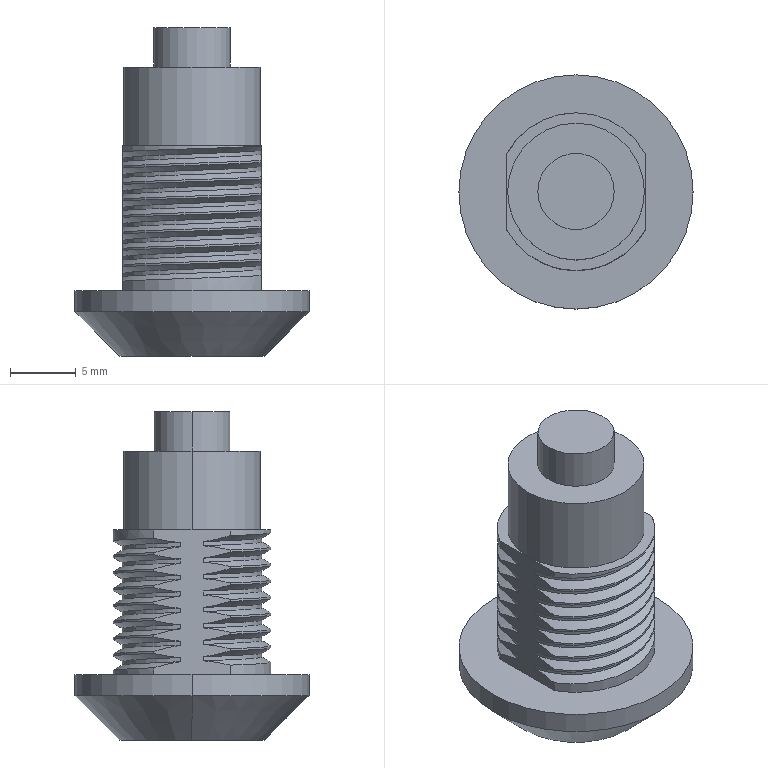Part | SolidWorks | features ICE 7, Chamfer 1, Extrusion 1, Fillet 1, SweepThread 1 | 1 solid | 106 faces | box 17.8 x 17.8 x 25 mm | volume 2223 mm3 | spline 48 | cylinder 37 | plane 16 | torus 3 | cone 2 | commonest cylinder face diameters 12 x18 1.5 x8 9 x3 5.5 x2 5.8 x2 10.4 x2